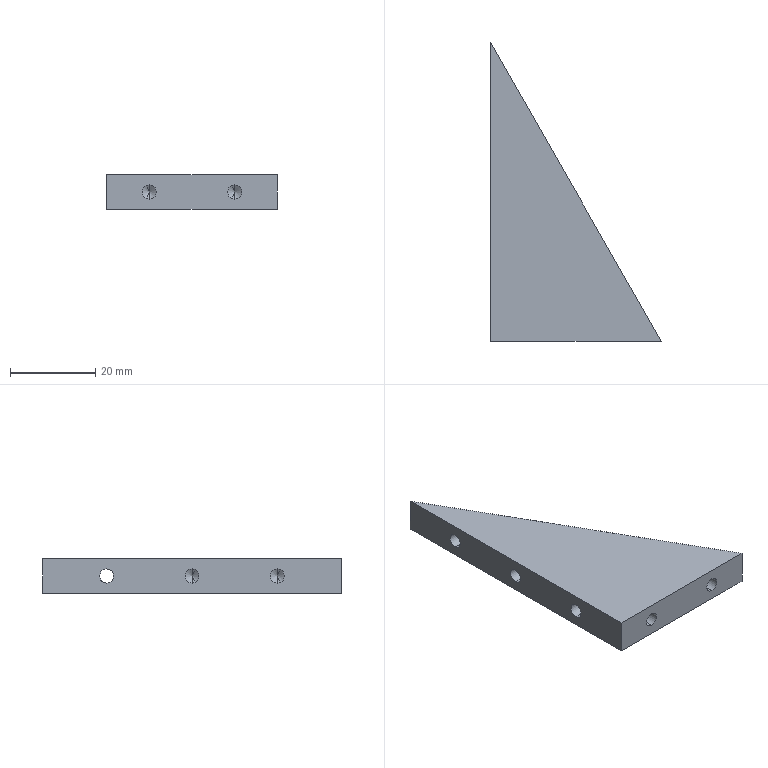Part | SolidWorks | features HoleWzd 2, Extrusion 1 | 1 solid | 23 faces | box 40 x 70 x 8 mm | volume 10705 mm3 | cylinder 10 | cone 8 | plane 5 | commonest cylinder face diameters 3.3 x10
STEP:
#1=CARTESIAN_POINT('',(10.,-23.,5.65));
#2=VERTEX_POINT('',#1);
#3=CARTESIAN_POINT('',(10.,-23.,2.35));
#4=VERTEX_POINT('',#3);
#5=CARTESIAN_POINT('',(10.,-23.,4.));
#6=DIRECTION('',(0.,-1.,0.));
#7=DIRECTION('',(0.,0.,-1.));
#8=AXIS2_PLACEMENT_3D('',#5,#6,#7);
#9=CIRCLE('',#8,1.65);
#10=EDGE_CURVE('',#2,#4,#9,.T.);
#11=ORIENTED_EDGE('',*,*,#10,.F.);
#12=CARTESIAN_POINT('',(10.,-35.,5.65));
#13=VERTEX_POINT('',#12);
#14=CARTESIAN_POINT('',(10.,-35.,5.65));
#15=DIRECTION('',(0.,-1.,0.));
#16=VECTOR('',#15,1000.);
#17=LINE('',#14,#16);
#18=EDGE_CURVE('',#2,#13,#17,.T.);
#19=ORIENTED_EDGE('',*,*,#18,.T.);
#20=CARTESIAN_POINT('',(10.,-35.,2.35));
#21=VERTEX_POINT('',#20);
#22=CARTESIAN_POINT('',(10.,-35.,4.));
#23=DIRECTION('',(0.,-1.,0.));
#24=DIRECTION('',(0.,0.,-1.));
#25=AXIS2_PLACEMENT_3D('',#22,#23,#24);
#26=CIRCLE('',#25,1.65);
#27=EDGE_CURVE('',#13,#21,#26,.T.);
#28=ORIENTED_EDGE('',*,*,#27,.T.);
#29=CARTESIAN_POINT('',(10.,-35.,2.35));
#30=DIRECTION('',(0.,-1.,0.));
#31=VECTOR('',#30,1000.);
#32=LINE('',#29,#31);
#33=EDGE_CURVE('',#4,#21,#32,.T.);
#34=ORIENTED_EDGE('',*,*,#33,.F.);
#35=EDGE_LOOP('',(#11,#19,#28,#34));
#36=FACE_OUTER_BOUND('',#35,.T.);
#37=CARTESIAN_POINT('',(10.,-35.,4.));
#38=DIRECTION('',(0.,-1.,0.));
#39=DIRECTION('',(0.,0.,-1.));
#40=AXIS2_PLACEMENT_3D('',#37,#38,#39);
#41=CYLINDRICAL_SURFACE('',#40,1.65);
#42=ADVANCED_FACE('',(#36),#41,.F.);
#43=CARTESIAN_POINT('',(10.,-22.009,4.));
#44=VERTEX_POINT('',#43);
#45=CARTESIAN_POINT('',(10.,-23.,2.35));
#46=DIRECTION('',(0.,-0.515,-0.8572));
#47=VECTOR('',#46,1000.);
#48=LINE('',#45,#47);
#49=EDGE_CURVE('',#44,#4,#48,.T.);
#50=ORIENTED_EDGE('',*,*,#49,.F.);
#51=CARTESIAN_POINT('',(10.,-23.,5.65));
#52=DIRECTION('',(0.,-0.515,0.8572));
#53=VECTOR('',#52,1000.);
#54=LINE('',#51,#53);
#55=EDGE_CURVE('',#44,#2,#54,.T.);
#56=ORIENTED_EDGE('',*,*,#55,.T.);
#57=ORIENTED_EDGE('',*,*,#10,.T.);
#58=EDGE_LOOP('',(#50,#56,#57));
#59=FACE_OUTER_BOUND('',#58,.T.);
#60=CARTESIAN_POINT('',(10.,-23.,4.));
#61=DIRECTION('',(0.,-1.,0.));
#62=DIRECTION('',(0.,0.,-1.));
#63=AXIS2_PLACEMENT_3D('',#60,#61,#62);
#64=CONICAL_SURFACE('',#63,1.65,1.03);
#65=ADVANCED_FACE('',(#59),#64,.F.);
#66=CARTESIAN_POINT('',(-10.,-23.,5.65));
#67=VERTEX_POINT('',#66);
#68=CARTESIAN_POINT('',(-10.,-23.,2.35));
#69=VERTEX_POINT('',#68);
#70=CARTESIAN_POINT('',(-10.,-23.,4.));
#71=DIRECTION('',(0.,-1.,0.));
#72=DIRECTION('',(0.,0.,-1.));
#73=AXIS2_PLACEMENT_3D('',#70,#71,#72);
#74=CIRCLE('',#73,1.65);
#75=EDGE_CURVE('',#67,#69,#74,.T.);
#76=ORIENTED_EDGE('',*,*,#75,.F.);
#77=CARTESIAN_POINT('',(-10.,-35.,5.65));
#78=VERTEX_POINT('',#77);
#79=CARTESIAN_POINT('',(-10.,-35.,5.65));
#80=DIRECTION('',(0.,-1.,0.));
#81=VECTOR('',#80,1000.);
#82=LINE('',#79,#81);
#83=EDGE_CURVE('',#67,#78,#82,.T.);
#84=ORIENTED_EDGE('',*,*,#83,.T.);
#85=CARTESIAN_POINT('',(-10.,-35.,2.35));
#86=VERTEX_POINT('',#85);
#87=CARTESIAN_POINT('',(-10.,-35.,4.));
#88=DIRECTION('',(0.,-1.,0.));
#89=DIRECTION('',(0.,0.,-1.));
#90=AXIS2_PLACEMENT_3D('',#87,#88,#89);
#91=CIRCLE('',#90,1.65);
#92=EDGE_CURVE('',#78,#86,#91,.T.);
#93=ORIENTED_EDGE('',*,*,#92,.T.);
#94=CARTESIAN_POINT('',(-10.,-35.,2.35));
#95=DIRECTION('',(0.,-1.,0.));
#96=VECTOR('',#95,1000.);
#97=LINE('',#94,#96);
#98=EDGE_CURVE('',#69,#86,#97,.T.);
#99=ORIENTED_EDGE('',*,*,#98,.F.);
#100=EDGE_LOOP('',(#76,#84,#93,#99));
#101=FACE_OUTER_BOUND('',#100,.T.);
#102=CARTESIAN_POINT('',(-10.,-35.,4.));
#103=DIRECTION('',(0.,-1.,0.));
#104=DIRECTION('',(0.,0.,-1.));
#105=AXIS2_PLACEMENT_3D('',#102,#103,#104);
#106=CYLINDRICAL_SURFACE('',#105,1.65);
#107=ADVANCED_FACE('',(#101),#106,.F.);
#108=CARTESIAN_POINT('',(-10.,-22.009,4.));
#109=VERTEX_POINT('',#108);
#110=CARTESIAN_POINT('',(-10.,-23.,2.35));
#111=DIRECTION('',(0.,-0.515,-0.8572));
#112=VECTOR('',#111,1000.);
#113=LINE('',#110,#112);
#114=EDGE_CURVE('',#109,#69,#113,.T.);
#115=ORIENTED_EDGE('',*,*,#114,.F.);
#116=CARTESIAN_POINT('',(-10.,-23.,5.65));
#117=DIRECTION('',(0.,-0.515,0.8572));
#118=VECTOR('',#117,1000.);
#119=LINE('',#116,#118);
#120=EDGE_CURVE('',#109,#67,#119,.T.);
#121=ORIENTED_EDGE('',*,*,#120,.T.);
#122=ORIENTED_EDGE('',*,*,#75,.T.);
#123=EDGE_LOOP('',(#115,#121,#122));
#124=FACE_OUTER_BOUND('',#123,.T.);
#125=CARTESIAN_POINT('',(-10.,-23.,4.));
#126=DIRECTION('',(0.,-1.,0.));
#127=DIRECTION('',(0.,0.,-1.));
#128=AXIS2_PLACEMENT_3D('',#125,#126,#127);
#129=CONICAL_SURFACE('',#128,1.65,1.03);
#130=ADVANCED_FACE('',(#124),#129,.F.);
#131=CARTESIAN_POINT('',(-8.,-20.,2.35));
#132=VERTEX_POINT('',#131);
#133=CARTESIAN_POINT('',(-8.,-20.,5.65));
#134=VERTEX_POINT('',#133);
#135=CARTESIAN_POINT('',(-8.,-20.,4.));
#136=DIRECTION('',(-1.,0.,0.));
#137=DIRECTION('',(0.,0.,1.));
#138=AXIS2_PLACEMENT_3D('',#135,#136,#137);
#139=CIRCLE('',#138,1.65);
#140=EDGE_CURVE('',#132,#134,#139,.T.);
#141=ORIENTED_EDGE('',*,*,#140,.F.);
#142=CARTESIAN_POINT('',(-20.,-20.,2.35));
#143=VERTEX_POINT('',#142);
#144=CARTESIAN_POINT('',(-20.,-20.,2.35));
#145=DIRECTION('',(-1.,0.,0.));
#146=VECTOR('',#145,1000.);
#147=LINE('',#144,#146);
#148=EDGE_CURVE('',#132,#143,#147,.T.);
#149=ORIENTED_EDGE('',*,*,#148,.T.);
#150=CARTESIAN_POINT('',(-20.,-20.,5.65));
#151=VERTEX_POINT('',#150);
#152=CARTESIAN_POINT('',(-20.,-20.,4.));
#153=DIRECTION('',(-1.,0.,0.));
#154=DIRECTION('',(0.,0.,1.));
#155=AXIS2_PLACEMENT_3D('',#152,#153,#154);
#156=CIRCLE('',#155,1.65);
#157=EDGE_CURVE('',#143,#151,#156,.T.);
#158=ORIENTED_EDGE('',*,*,#157,.T.);
#159=CARTESIAN_POINT('',(-20.,-20.,5.65));
#160=DIRECTION('',(-1.,0.,0.));
#161=VECTOR('',#160,1000.);
#162=LINE('',#159,#161);
#163=EDGE_CURVE('',#134,#151,#162,.T.);
#164=ORIENTED_EDGE('',*,*,#163,.F.);
#165=EDGE_LOOP('',(#141,#149,#158,#164));
#166=FACE_OUTER_BOUND('',#165,.T.);
#167=CARTESIAN_POINT('',(-20.,-20.,4.));
#168=DIRECTION('',(-1.,0.,0.));
#169=DIRECTION('',(0.,0.,1.));
#170=AXIS2_PLACEMENT_3D('',#167,#168,#169);
#171=CYLINDRICAL_SURFACE('',#170,1.65);
#172=ADVANCED_FACE('',(#166),#171,.F.);
#173=CARTESIAN_POINT('',(-7.009,-20.,4.));
#174=VERTEX_POINT('',#173);
#175=CARTESIAN_POINT('',(-8.,-20.,5.65));
#176=DIRECTION('',(-0.515,0.,0.8572));
#177=VECTOR('',#176,1000.);
#178=LINE('',#175,#177);
#179=EDGE_CURVE('',#174,#134,#178,.T.);
#180=ORIENTED_EDGE('',*,*,#179,.F.);
#181=CARTESIAN_POINT('',(-8.,-20.,2.35));
#182=DIRECTION('',(-0.515,0.,-0.8572));
#183=VECTOR('',#182,1000.);
#184=LINE('',#181,#183);
#185=EDGE_CURVE('',#174,#132,#184,.T.);
#186=ORIENTED_EDGE('',*,*,#185,.T.);
#187=ORIENTED_EDGE('',*,*,#140,.T.);
#188=EDGE_LOOP('',(#180,#186,#187));
#189=FACE_OUTER_BOUND('',#188,.T.);
#190=CARTESIAN_POINT('',(-8.,-20.,4.));
#191=DIRECTION('',(-1.,0.,0.));
#192=DIRECTION('',(0.,0.,1.));
#193=AXIS2_PLACEMENT_3D('',#190,#191,#192);
#194=CONICAL_SURFACE('',#193,1.65,1.03);
#195=ADVANCED_FACE('',(#189),#194,.F.);
#196=CARTESIAN_POINT('',(-8.,0.,2.35));
#197=VERTEX_POINT('',#196);
#198=CARTESIAN_POINT('',(-8.,0.,5.65));
#199=VERTEX_POINT('',#198);
#200=CARTESIAN_POINT('',(-8.,0.,4.));
#201=DIRECTION('',(-1.,0.,0.));
#202=DIRECTION('',(0.,0.,1.));
#203=AXIS2_PLACEMENT_3D('',#200,#201,#202);
#204=CIRCLE('',#203,1.65);
#205=EDGE_CURVE('',#197,#199,#204,.T.);
#206=ORIENTED_EDGE('',*,*,#205,.F.);
#207=CARTESIAN_POINT('',(-20.,0.,2.35));
#208=VERTEX_POINT('',#207);
#209=CARTESIAN_POINT('',(-20.,0.,2.35));
#210=DIRECTION('',(-1.,0.,0.));
#211=VECTOR('',#210,1000.);
#212=LINE('',#209,#211);
#213=EDGE_CURVE('',#197,#208,#212,.T.);
#214=ORIENTED_EDGE('',*,*,#213,.T.);
#215=CARTESIAN_POINT('',(-20.,0.,5.65));
#216=VERTEX_POINT('',#215);
#217=CARTESIAN_POINT('',(-20.,0.,4.));
#218=DIRECTION('',(-1.,0.,0.));
#219=DIRECTION('',(0.,0.,1.));
#220=AXIS2_PLACEMENT_3D('',#217,#218,#219);
#221=CIRCLE('',#220,1.65);
#222=EDGE_CURVE('',#208,#216,#221,.T.);
#223=ORIENTED_EDGE('',*,*,#222,.T.);
#224=CARTESIAN_POINT('',(-20.,0.,5.65));
#225=DIRECTION('',(-1.,0.,0.));
#226=VECTOR('',#225,1000.);
#227=LINE('',#224,#226);
#228=EDGE_CURVE('',#199,#216,#227,.T.);
#229=ORIENTED_EDGE('',*,*,#228,.F.);
#230=EDGE_LOOP('',(#206,#214,#223,#229));
#231=FACE_OUTER_BOUND('',#230,.T.);
#232=CARTESIAN_POINT('',(-20.,0.,4.));
#233=DIRECTION('',(-1.,0.,0.));
#234=DIRECTION('',(0.,0.,1.));
#235=AXIS2_PLACEMENT_3D('',#232,#233,#234);
#236=CYLINDRICAL_SURFACE('',#235,1.65);
#237=ADVANCED_FACE('',(#231),#236,.F.);
#238=CARTESIAN_POINT('',(-7.009,0.,4.));
#239=VERTEX_POINT('',#238);
#240=CARTESIAN_POINT('',(-8.,0.,5.65));
#241=DIRECTION('',(-0.515,0.,0.8572));
#242=VECTOR('',#241,1000.);
#243=LINE('',#240,#242);
#244=EDGE_CURVE('',#239,#199,#243,.T.);
#245=ORIENTED_EDGE('',*,*,#244,.F.);
#246=CARTESIAN_POINT('',(-8.,0.,2.35));
#247=DIRECTION('',(-0.515,0.,-0.8572));
#248=VECTOR('',#247,1000.);
#249=LINE('',#246,#248);
#250=EDGE_CURVE('',#239,#197,#249,.T.);
#251=ORIENTED_EDGE('',*,*,#250,.T.);
#252=ORIENTED_EDGE('',*,*,#205,.T.);
#253=EDGE_LOOP('',(#245,#251,#252));
#254=FACE_OUTER_BOUND('',#253,.T.);
#255=CARTESIAN_POINT('',(-8.,0.,4.));
#256=DIRECTION('',(-1.,0.,0.));
#257=DIRECTION('',(0.,0.,1.));
#258=AXIS2_PLACEMENT_3D('',#255,#256,#257);
#259=CONICAL_SURFACE('',#258,1.65,1.03);
#260=ADVANCED_FACE('',(#254),#259,.F.);
#261=CARTESIAN_POINT('',(-11.429,20.,2.35));
#262=VERTEX_POINT('',#261);
#263=CARTESIAN_POINT('',(-11.429,20.,5.65));
#264=VERTEX_POINT('',#263);
#265=CARTESIAN_POINT('',(-11.429,20.,2.35));
#266=CARTESIAN_POINT('',(-9.543,16.7,2.35));
#267=CARTESIAN_POINT('',(-9.543,16.7,5.65));
#268=CARTESIAN_POINT('',(-11.429,20.,5.65));
#269=(BOUNDED_CURVE()B_SPLINE_CURVE(3,(#265,#266,#267,#268),.UNSPECIFIED.,.F.,.F.)B_SPLINE_CURVE_WITH_KNOTS((4,4),(1.571,4.712),.UNSPECIFIED.)CURVE()GEOMETRIC_REPRESENTATION_ITEM()RATIONAL_B_SPLINE_CURVE((1.,0.3333,0.3333,1.))REPRESENTATION_ITEM(''));
#270=EDGE_CURVE('',#262,#264,#269,.T.);
#271=ORIENTED_EDGE('',*,*,#270,.F.);
#272=CARTESIAN_POINT('',(-20.,20.,2.35));
#273=VERTEX_POINT('',#272);
#274=CARTESIAN_POINT('',(-20.,20.,2.35));
#275=DIRECTION('',(-1.,0.,0.));
#276=VECTOR('',#275,1000.);
#277=LINE('',#274,#276);
#278=EDGE_CURVE('',#262,#273,#277,.T.);
#279=ORIENTED_EDGE('',*,*,#278,.T.);
#280=CARTESIAN_POINT('',(-20.,20.,5.65));
#281=VERTEX_POINT('',#280);
#282=CARTESIAN_POINT('',(-20.,20.,4.));
#283=DIRECTION('',(-1.,0.,0.));
#284=DIRECTION('',(0.,0.,1.));
#285=AXIS2_PLACEMENT_3D('',#282,#283,#284);
#286=CIRCLE('',#285,1.65);
#287=EDGE_CURVE('',#273,#281,#286,.T.);
#288=ORIENTED_EDGE('',*,*,#287,.T.);
#289=CARTESIAN_POINT('',(-20.,20.,5.65));
#290=DIRECTION('',(-1.,0.,0.));
#291=VECTOR('',#290,1000.);
#292=LINE('',#289,#291);
#293=EDGE_CURVE('',#264,#281,#292,.T.);
#294=ORIENTED_EDGE('',*,*,#293,.F.);
#295=EDGE_LOOP('',(#271,#279,#288,#294));
#296=FACE_OUTER_BOUND('',#295,.T.);
#297=CARTESIAN_POINT('',(-20.,20.,4.));
#298=DIRECTION('',(-1.,0.,0.));
#299=DIRECTION('',(0.,0.,1.));
#300=AXIS2_PLACEMENT_3D('',#297,#298,#299);
#301=CYLINDRICAL_SURFACE('',#300,1.65);
#302=ADVANCED_FACE('',(#296),#301,.F.);
#303=CARTESIAN_POINT('',(-20.,-20.,4.));
#304=DIRECTION('',(-1.,0.,0.));
#305=DIRECTION('',(0.,0.,1.));
#306=AXIS2_PLACEMENT_3D('',#303,#304,#305);
#307=CIRCLE('',#306,1.65);
#308=EDGE_CURVE('',#151,#143,#307,.T.);
#309=ORIENTED_EDGE('',*,*,#308,.F.);
#310=ORIENTED_EDGE('',*,*,#157,.F.);
#311=EDGE_LOOP('',(#309,#310));
#312=FACE_BOUND('',#311,.T.);
#313=CARTESIAN_POINT('',(-20.,0.,4.));
#314=DIRECTION('',(-1.,0.,0.));
#315=DIRECTION('',(0.,0.,1.));
#316=AXIS2_PLACEMENT_3D('',#313,#314,#315);
#317=CIRCLE('',#316,1.65);
#318=EDGE_CURVE('',#216,#208,#317,.T.);
#319=ORIENTED_EDGE('',*,*,#318,.F.);
#320=ORIENTED_EDGE('',*,*,#222,.F.);
#321=EDGE_LOOP('',(#319,#320));
#322=FACE_BOUND('',#321,.T.);
#323=CARTESIAN_POINT('',(-20.,20.,4.));
#324=DIRECTION('',(-1.,0.,0.));
#325=DIRECTION('',(0.,0.,1.));
#326=AXIS2_PLACEMENT_3D('',#323,#324,#325);
#327=CIRCLE('',#326,1.65);
#328=EDGE_CURVE('',#281,#273,#327,.T.);
#329=ORIENTED_EDGE('',*,*,#328,.F.);
#330=ORIENTED_EDGE('',*,*,#287,.F.);
#331=EDGE_LOOP('',(#329,#330));
#332=FACE_BOUND('',#331,.T.);
#333=CARTESIAN_POINT('',(-20.,35.,0.));
#334=VERTEX_POINT('',#333);
#335=CARTESIAN_POINT('',(-20.,-35.,0.));
#336=VERTEX_POINT('',#335);
#337=CARTESIAN_POINT('',(-20.,35.,0.));
#338=DIRECTION('',(0.,-1.,0.));
#339=VECTOR('',#338,1000.);
#340=LINE('',#337,#339);
#341=EDGE_CURVE('',#334,#336,#340,.T.);
#342=ORIENTED_EDGE('',*,*,#341,.T.);
#343=CARTESIAN_POINT('',(-20.,-35.,8.));
#344=VERTEX_POINT('',#343);
#345=CARTESIAN_POINT('',(-20.,-35.,8.));
#346=DIRECTION('',(0.,0.,-1.));
#347=VECTOR('',#346,1000.);
#348=LINE('',#345,#347);
#349=EDGE_CURVE('',#344,#336,#348,.T.);
#350=ORIENTED_EDGE('',*,*,#349,.F.);
#351=CARTESIAN_POINT('',(-20.,35.,8.));
#352=VERTEX_POINT('',#351);
#353=CARTESIAN_POINT('',(-20.,35.,8.));
#354=DIRECTION('',(0.,-1.,0.));
#355=VECTOR('',#354,1000.);
#356=LINE('',#353,#355);
#357=EDGE_CURVE('',#352,#344,#356,.T.);
#358=ORIENTED_EDGE('',*,*,#357,.F.);
#359=CARTESIAN_POINT('',(-20.,35.,8.));
#360=DIRECTION('',(0.,0.,-1.));
#361=VECTOR('',#360,1000.);
#362=LINE('',#359,#361);
#363=EDGE_CURVE('',#352,#334,#362,.T.);
#364=ORIENTED_EDGE('',*,*,#363,.T.);
#365=EDGE_LOOP('',(#342,#350,#358,#364));
#366=FACE_OUTER_BOUND('',#365,.T.);
#367=CARTESIAN_POINT('',(-20.,35.,8.));
#368=DIRECTION('',(1.,0.,0.));
#369=DIRECTION('',(0.,1.,0.));
#370=AXIS2_PLACEMENT_3D('',#367,#368,#369);
#371=PLANE('',#370);
#372=ADVANCED_FACE('',(#312,#322,#332,#366),#371,.F.);
#373=CARTESIAN_POINT('',(10.,-35.,4.));
#374=DIRECTION('',(0.,-1.,0.));
#375=DIRECTION('',(0.,0.,-1.));
#376=AXIS2_PLACEMENT_3D('',#373,#374,#375);
#377=CIRCLE('',#376,1.65);
#378=EDGE_CURVE('',#21,#13,#377,.T.);
#379=ORIENTED_EDGE('',*,*,#378,.F.);
#380=ORIENTED_EDGE('',*,*,#27,.F.);
#381=EDGE_LOOP('',(#379,#380));
#382=FACE_BOUND('',#381,.T.);
#383=CARTESIAN_POINT('',(-10.,-35.,4.));
#384=DIRECTION('',(0.,-1.,0.));
#385=DIRECTION('',(0.,0.,-1.));
#386=AXIS2_PLACEMENT_3D('',#383,#384,#385);
#387=CIRCLE('',#386,1.65);
#388=EDGE_CURVE('',#86,#78,#387,.T.);
#389=ORIENTED_EDGE('',*,*,#388,.F.);
#390=ORIENTED_EDGE('',*,*,#92,.F.);
#391=EDGE_LOOP('',(#389,#390));
#392=FACE_BOUND('',#391,.T.);
#393=CARTESIAN_POINT('',(20.,-35.,0.));
#394=VERTEX_POINT('',#393);
#395=CARTESIAN_POINT('',(-20.,-35.,0.));
#396=DIRECTION('',(1.,0.,0.));
#397=VECTOR('',#396,1000.);
#398=LINE('',#395,#397);
#399=EDGE_CURVE('',#336,#394,#398,.T.);
#400=ORIENTED_EDGE('',*,*,#399,.T.);
#401=CARTESIAN_POINT('',(20.,-35.,8.));
#402=VERTEX_POINT('',#401);
#403=CARTESIAN_POINT('',(20.,-35.,8.));
#404=DIRECTION('',(0.,0.,-1.));
#405=VECTOR('',#404,1000.);
#406=LINE('',#403,#405);
#407=EDGE_CURVE('',#402,#394,#406,.T.);
#408=ORIENTED_EDGE('',*,*,#407,.F.);
#409=CARTESIAN_POINT('',(-20.,-35.,8.));
#410=DIRECTION('',(1.,0.,0.));
#411=VECTOR('',#410,1000.);
#412=LINE('',#409,#411);
#413=EDGE_CURVE('',#344,#402,#412,.T.);
#414=ORIENTED_EDGE('',*,*,#413,.F.);
#415=ORIENTED_EDGE('',*,*,#349,.T.);
#416=EDGE_LOOP('',(#400,#408,#414,#415));
#417=FACE_OUTER_BOUND('',#416,.T.);
#418=CARTESIAN_POINT('',(-20.,-35.,8.));
#419=DIRECTION('',(0.,1.,0.));
#420=DIRECTION('',(0.,0.,1.));
#421=AXIS2_PLACEMENT_3D('',#418,#419,#420);
#422=PLANE('',#421);
#423=ADVANCED_FACE('',(#382,#392,#417),#422,.F.);
#424=CARTESIAN_POINT('',(-11.429,20.,5.65));
#425=CARTESIAN_POINT('',(-13.314,23.3,5.65));
#426=CARTESIAN_POINT('',(-13.314,23.3,2.35));
#427=CARTESIAN_POINT('',(-11.429,20.,2.35));
#428=(BOUNDED_CURVE()B_SPLINE_CURVE(3,(#424,#425,#426,#427),.UNSPECIFIED.,.F.,.F.)B_SPLINE_CURVE_WITH_KNOTS((4,4),(4.712,7.854),.UNSPECIFIED.)CURVE()GEOMETRIC_REPRESENTATION_ITEM()RATIONAL_B_SPLINE_CURVE((1.,0.3333,0.3333,1.))REPRESENTATION_ITEM(''));
#429=EDGE_CURVE('',#264,#262,#428,.T.);
#430=ORIENTED_EDGE('',*,*,#429,.T.);
#431=ORIENTED_EDGE('',*,*,#270,.T.);
#432=EDGE_LOOP('',(#430,#431));
#433=FACE_BOUND('',#432,.T.);
#434=CARTESIAN_POINT('',(20.,-35.,0.));
#435=DIRECTION('',(-0.4961,0.8682,0.));
#436=VECTOR('',#435,1000.);
#437=LINE('',#434,#436);
#438=EDGE_CURVE('',#394,#334,#437,.T.);
#439=ORIENTED_EDGE('',*,*,#438,.T.);
#440=ORIENTED_EDGE('',*,*,#363,.F.);
#441=CARTESIAN_POINT('',(20.,-35.,8.));
#442=DIRECTION('',(-0.4961,0.8682,0.));
#443=VECTOR('',#442,1000.);
#444=LINE('',#441,#443);
#445=EDGE_CURVE('',#402,#352,#444,.T.);
#446=ORIENTED_EDGE('',*,*,#445,.F.);
#447=ORIENTED_EDGE('',*,*,#407,.T.);
#448=EDGE_LOOP('',(#439,#440,#446,#447));
#449=FACE_OUTER_BOUND('',#448,.T.);
#450=CARTESIAN_POINT('',(20.,-35.,8.));
#451=DIRECTION('',(-0.8682,-0.4961,0.));
#452=DIRECTION('',(0.4961,-0.8682,0.));
#453=AXIS2_PLACEMENT_3D('',#450,#451,#452);
#454=PLANE('',#453);
#455=ADVANCED_FACE('',(#433,#449),#454,.F.);
#456=ORIENTED_EDGE('',*,*,#357,.T.);
#457=ORIENTED_EDGE('',*,*,#413,.T.);
#458=ORIENTED_EDGE('',*,*,#445,.T.);
#459=EDGE_LOOP('',(#456,#457,#458));
#460=FACE_OUTER_BOUND('',#459,.T.);
#461=CARTESIAN_POINT('',(0.,0.,8.));
#462=DIRECTION('',(0.,0.,1.));
#463=DIRECTION('',(1.,0.,0.));
#464=AXIS2_PLACEMENT_3D('',#461,#462,#463);
#465=PLANE('',#464);
#466=ADVANCED_FACE('',(#460),#465,.T.);
#467=ORIENTED_EDGE('',*,*,#341,.F.);
#468=ORIENTED_EDGE('',*,*,#438,.F.);
#469=ORIENTED_EDGE('',*,*,#399,.F.);
#470=EDGE_LOOP('',(#467,#468,#469));
#471=FACE_OUTER_BOUND('',#470,.T.);
#472=CARTESIAN_POINT('',(0.,0.,0.));
#473=DIRECTION('',(0.,0.,1.));
#474=DIRECTION('',(1.,0.,0.));
#475=AXIS2_PLACEMENT_3D('',#472,#473,#474);
#476=PLANE('',#475);
#477=ADVANCED_FACE('',(#471),#476,.F.);
#478=ORIENTED_EDGE('',*,*,#278,.F.);
#479=ORIENTED_EDGE('',*,*,#429,.F.);
#480=ORIENTED_EDGE('',*,*,#293,.T.);
#481=ORIENTED_EDGE('',*,*,#328,.T.);
#482=EDGE_LOOP('',(#478,#479,#480,#481));
#483=FACE_OUTER_BOUND('',#482,.T.);
#484=CARTESIAN_POINT('',(-20.,20.,4.));
#485=DIRECTION('',(-1.,0.,0.));
#486=DIRECTION('',(0.,0.,1.));
#487=AXIS2_PLACEMENT_3D('',#484,#485,#486);
#488=CYLINDRICAL_SURFACE('',#487,1.65);
#489=ADVANCED_FACE('',(#483),#488,.F.);
#490=ORIENTED_EDGE('',*,*,#250,.F.);
#491=ORIENTED_EDGE('',*,*,#244,.T.);
#492=CARTESIAN_POINT('',(-8.,0.,4.));
#493=DIRECTION('',(-1.,0.,0.));
#494=DIRECTION('',(0.,0.,1.));
#495=AXIS2_PLACEMENT_3D('',#492,#493,#494);
#496=CIRCLE('',#495,1.65);
#497=EDGE_CURVE('',#199,#197,#496,.T.);
#498=ORIENTED_EDGE('',*,*,#497,.T.);
#499=EDGE_LOOP('',(#490,#491,#498));
#500=FACE_OUTER_BOUND('',#499,.T.);
#501=CARTESIAN_POINT('',(-8.,0.,4.));
#502=DIRECTION('',(-1.,0.,0.));
#503=DIRECTION('',(0.,0.,1.));
#504=AXIS2_PLACEMENT_3D('',#501,#502,#503);
#505=CONICAL_SURFACE('',#504,1.65,1.03);
#506=ADVANCED_FACE('',(#500),#505,.F.);
#507=ORIENTED_EDGE('',*,*,#213,.F.);
#508=ORIENTED_EDGE('',*,*,#497,.F.);
#509=ORIENTED_EDGE('',*,*,#228,.T.);
#510=ORIENTED_EDGE('',*,*,#318,.T.);
#511=EDGE_LOOP('',(#507,#508,#509,#510));
#512=FACE_OUTER_BOUND('',#511,.T.);
#513=CARTESIAN_POINT('',(-20.,0.,4.));
#514=DIRECTION('',(-1.,0.,0.));
#515=DIRECTION('',(0.,0.,1.));
#516=AXIS2_PLACEMENT_3D('',#513,#514,#515);
#517=CYLINDRICAL_SURFACE('',#516,1.65);
#518=ADVANCED_FACE('',(#512),#517,.F.);
#519=ORIENTED_EDGE('',*,*,#185,.F.);
#520=ORIENTED_EDGE('',*,*,#179,.T.);
#521=CARTESIAN_POINT('',(-8.,-20.,4.));
#522=DIRECTION('',(-1.,0.,0.));
#523=DIRECTION('',(0.,0.,1.));
#524=AXIS2_PLACEMENT_3D('',#521,#522,#523);
#525=CIRCLE('',#524,1.65);
#526=EDGE_CURVE('',#134,#132,#525,.T.);
#527=ORIENTED_EDGE('',*,*,#526,.T.);
#528=EDGE_LOOP('',(#519,#520,#527));
#529=FACE_OUTER_BOUND('',#528,.T.);
#530=CARTESIAN_POINT('',(-8.,-20.,4.));
#531=DIRECTION('',(-1.,0.,0.));
#532=DIRECTION('',(0.,0.,1.));
#533=AXIS2_PLACEMENT_3D('',#530,#531,#532);
#534=CONICAL_SURFACE('',#533,1.65,1.03);
#535=ADVANCED_FACE('',(#529),#534,.F.);
#536=ORIENTED_EDGE('',*,*,#148,.F.);
#537=ORIENTED_EDGE('',*,*,#526,.F.);
#538=ORIENTED_EDGE('',*,*,#163,.T.);
#539=ORIENTED_EDGE('',*,*,#308,.T.);
#540=EDGE_LOOP('',(#536,#537,#538,#539));
#541=FACE_OUTER_BOUND('',#540,.T.);
#542=CARTESIAN_POINT('',(-20.,-20.,4.));
#543=DIRECTION('',(-1.,0.,0.));
#544=DIRECTION('',(0.,0.,1.));
#545=AXIS2_PLACEMENT_3D('',#542,#543,#544);
#546=CYLINDRICAL_SURFACE('',#545,1.65);
#547=ADVANCED_FACE('',(#541),#546,.F.);
#548=ORIENTED_EDGE('',*,*,#120,.F.);
#549=ORIENTED_EDGE('',*,*,#114,.T.);
#550=CARTESIAN_POINT('',(-10.,-23.,4.));
#551=DIRECTION('',(0.,-1.,0.));
#552=DIRECTION('',(0.,0.,-1.));
#553=AXIS2_PLACEMENT_3D('',#550,#551,#552);
#554=CIRCLE('',#553,1.65);
#555=EDGE_CURVE('',#69,#67,#554,.T.);
#556=ORIENTED_EDGE('',*,*,#555,.T.);
#557=EDGE_LOOP('',(#548,#549,#556));
#558=FACE_OUTER_BOUND('',#557,.T.);
#559=CARTESIAN_POINT('',(-10.,-23.,4.));
#560=DIRECTION('',(0.,-1.,0.));
#561=DIRECTION('',(0.,0.,-1.));
#562=AXIS2_PLACEMENT_3D('',#559,#560,#561);
#563=CONICAL_SURFACE('',#562,1.65,1.03);
#564=ADVANCED_FACE('',(#558),#563,.F.);
#565=ORIENTED_EDGE('',*,*,#83,.F.);
#566=ORIENTED_EDGE('',*,*,#555,.F.);
#567=ORIENTED_EDGE('',*,*,#98,.T.);
#568=ORIENTED_EDGE('',*,*,#388,.T.);
#569=EDGE_LOOP('',(#565,#566,#567,#568));
#570=FACE_OUTER_BOUND('',#569,.T.);
#571=CARTESIAN_POINT('',(-10.,-35.,4.));
#572=DIRECTION('',(0.,-1.,0.));
#573=DIRECTION('',(0.,0.,-1.));
#574=AXIS2_PLACEMENT_3D('',#571,#572,#573);
#575=CYLINDRICAL_SURFACE('',#574,1.65);
#576=ADVANCED_FACE('',(#570),#575,.F.);
#577=ORIENTED_EDGE('',*,*,#55,.F.);
#578=ORIENTED_EDGE('',*,*,#49,.T.);
#579=CARTESIAN_POINT('',(10.,-23.,4.));
#580=DIRECTION('',(0.,-1.,0.));
#581=DIRECTION('',(0.,0.,-1.));
#582=AXIS2_PLACEMENT_3D('',#579,#580,#581);
#583=CIRCLE('',#582,1.65);
#584=EDGE_CURVE('',#4,#2,#583,.T.);
#585=ORIENTED_EDGE('',*,*,#584,.T.);
#586=EDGE_LOOP('',(#577,#578,#585));
#587=FACE_OUTER_BOUND('',#586,.T.);
#588=CARTESIAN_POINT('',(10.,-23.,4.));
#589=DIRECTION('',(0.,-1.,0.));
#590=DIRECTION('',(0.,0.,-1.));
#591=AXIS2_PLACEMENT_3D('',#588,#589,#590);
#592=CONICAL_SURFACE('',#591,1.65,1.03);
#593=ADVANCED_FACE('',(#587),#592,.F.);
#594=ORIENTED_EDGE('',*,*,#18,.F.);
#595=ORIENTED_EDGE('',*,*,#584,.F.);
#596=ORIENTED_EDGE('',*,*,#33,.T.);
#597=ORIENTED_EDGE('',*,*,#378,.T.);
#598=EDGE_LOOP('',(#594,#595,#596,#597));
#599=FACE_OUTER_BOUND('',#598,.T.);
#600=CARTESIAN_POINT('',(10.,-35.,4.));
#601=DIRECTION('',(0.,-1.,0.));
#602=DIRECTION('',(0.,0.,-1.));
#603=AXIS2_PLACEMENT_3D('',#600,#601,#602);
#604=CYLINDRICAL_SURFACE('',#603,1.65);
#605=ADVANCED_FACE('',(#599),#604,.F.);
#606=CLOSED_SHELL('',(#42,#65,#107,#130,#172,#195,#237,#260,#302,#372,#423,#455,#466,#477,#489,#506,#518,#535,#547,#564,#576,#593,#605));
#607=MANIFOLD_SOLID_BREP('',#606);
#608=CARTESIAN_POINT('',(0.,0.,0.));
#609=DIRECTION('',(0.,0.,1.));
#610=DIRECTION('',(1.,0.,0.));
#611=AXIS2_PLACEMENT_3D('',#608,#609,#610);
#612=(LENGTH_UNIT()NAMED_UNIT(*)SI_UNIT(.MILLI.,.METRE.));
#613=UNCERTAINTY_MEASURE_WITH_UNIT(LENGTH_MEASURE(0.00001),#612,'','');
#614=(NAMED_UNIT(*)PLANE_ANGLE_UNIT()SI_UNIT($,.RADIAN.));
#615=(NAMED_UNIT(*)SI_UNIT($,.STERADIAN.)SOLID_ANGLE_UNIT());
#616=(GEOMETRIC_REPRESENTATION_CONTEXT(3)GLOBAL_UNCERTAINTY_ASSIGNED_CONTEXT((#613))GLOBAL_UNIT_ASSIGNED_CONTEXT((#612,#614,#615))REPRESENTATION_CONTEXT('',''));
#617=ADVANCED_BREP_SHAPE_REPRESENTATION('',(#607,#611),#616);